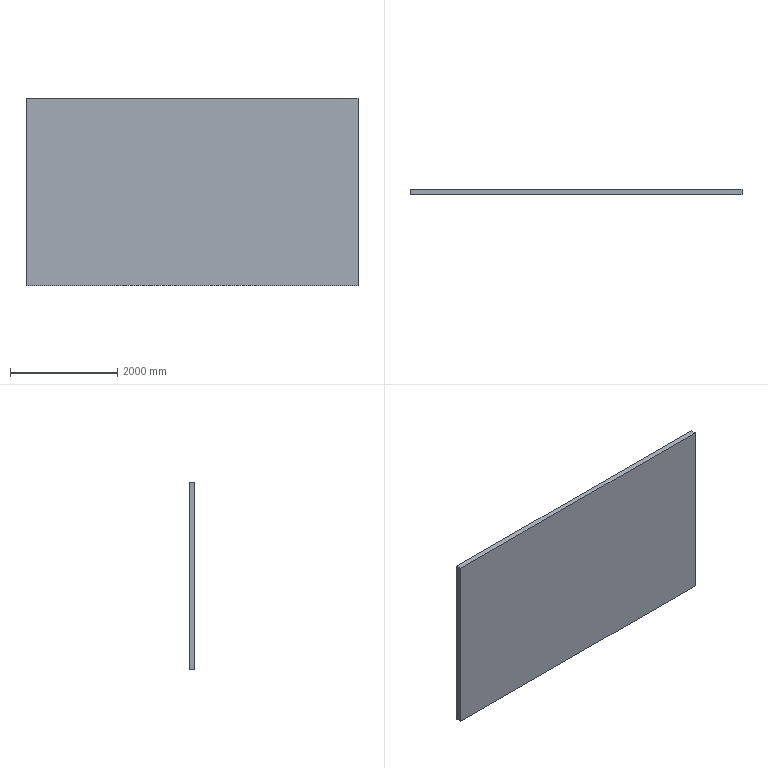Part | SolidWorks | features Cut 1, Extrusion 1 | 1 solid | 6 faces | box 6200 x 100 x 3500 mm | volume 2170000000 mm3 | plane 6
STEP:
#1=CARTESIAN_POINT('',(2800.,0.,-2400.));
#2=VERTEX_POINT('',#1);
#3=CARTESIAN_POINT('',(2800.,100.,-2400.));
#4=VERTEX_POINT('',#3);
#5=CARTESIAN_POINT('',(2800.,0.,-2400.));
#6=DIRECTION('',(0.,1.,0.));
#7=VECTOR('',#6,1000.);
#8=LINE('',#5,#7);
#9=EDGE_CURVE('',#2,#4,#8,.T.);
#10=ORIENTED_EDGE('',*,*,#9,.F.);
#11=CARTESIAN_POINT('',(-3400.,0.,-2400.));
#12=VERTEX_POINT('',#11);
#13=CARTESIAN_POINT('',(-3400.,0.,-2400.));
#14=DIRECTION('',(-1.,0.,0.));
#15=VECTOR('',#14,1000.);
#16=LINE('',#13,#15);
#17=EDGE_CURVE('',#2,#12,#16,.T.);
#18=ORIENTED_EDGE('',*,*,#17,.T.);
#19=CARTESIAN_POINT('',(-3400.,100.,-2400.));
#20=VERTEX_POINT('',#19);
#21=CARTESIAN_POINT('',(-3400.,100.,-2400.));
#22=DIRECTION('',(0.,-1.,0.));
#23=VECTOR('',#22,1000.);
#24=LINE('',#21,#23);
#25=EDGE_CURVE('',#20,#12,#24,.T.);
#26=ORIENTED_EDGE('',*,*,#25,.F.);
#27=CARTESIAN_POINT('',(-3400.,100.,-2400.));
#28=DIRECTION('',(-1.,0.,0.));
#29=VECTOR('',#28,1000.);
#30=LINE('',#27,#29);
#31=EDGE_CURVE('',#4,#20,#30,.T.);
#32=ORIENTED_EDGE('',*,*,#31,.F.);
#33=EDGE_LOOP('',(#10,#18,#26,#32));
#34=FACE_OUTER_BOUND('',#33,.T.);
#35=CARTESIAN_POINT('',(-3400.,100.,-2400.));
#36=DIRECTION('',(0.,0.,1.));
#37=DIRECTION('',(1.,0.,0.));
#38=AXIS2_PLACEMENT_3D('',#35,#36,#37);
#39=PLANE('',#38);
#40=ADVANCED_FACE('',(#34),#39,.F.);
#41=CARTESIAN_POINT('',(-3400.,0.,1100.));
#42=VERTEX_POINT('',#41);
#43=CARTESIAN_POINT('',(-3400.,100.,1100.));
#44=VERTEX_POINT('',#43);
#45=CARTESIAN_POINT('',(-3400.,0.,1100.));
#46=DIRECTION('',(0.,1.,0.));
#47=VECTOR('',#46,1000.);
#48=LINE('',#45,#47);
#49=EDGE_CURVE('',#42,#44,#48,.T.);
#50=ORIENTED_EDGE('',*,*,#49,.T.);
#51=CARTESIAN_POINT('',(-3400.,100.,-2400.));
#52=DIRECTION('',(0.,0.,1.));
#53=VECTOR('',#52,1000.);
#54=LINE('',#51,#53);
#55=EDGE_CURVE('',#20,#44,#54,.T.);
#56=ORIENTED_EDGE('',*,*,#55,.F.);
#57=ORIENTED_EDGE('',*,*,#25,.T.);
#58=CARTESIAN_POINT('',(-3400.,0.,-2400.));
#59=DIRECTION('',(0.,0.,1.));
#60=VECTOR('',#59,1000.);
#61=LINE('',#58,#60);
#62=EDGE_CURVE('',#12,#42,#61,.T.);
#63=ORIENTED_EDGE('',*,*,#62,.T.);
#64=EDGE_LOOP('',(#50,#56,#57,#63));
#65=FACE_OUTER_BOUND('',#64,.T.);
#66=CARTESIAN_POINT('',(-3400.,100.,-2400.));
#67=DIRECTION('',(1.,0.,0.));
#68=DIRECTION('',(0.,0.,-1.));
#69=AXIS2_PLACEMENT_3D('',#66,#67,#68);
#70=PLANE('',#69);
#71=ADVANCED_FACE('',(#65),#70,.F.);
#72=CARTESIAN_POINT('',(2800.,100.,1100.));
#73=VERTEX_POINT('',#72);
#74=CARTESIAN_POINT('',(-3400.,100.,1100.));
#75=DIRECTION('',(1.,0.,0.));
#76=VECTOR('',#75,1000.);
#77=LINE('',#74,#76);
#78=EDGE_CURVE('',#44,#73,#77,.T.);
#79=ORIENTED_EDGE('',*,*,#78,.T.);
#80=CARTESIAN_POINT('',(2800.,100.,-2400.));
#81=DIRECTION('',(0.,0.,-1.));
#82=VECTOR('',#81,1000.);
#83=LINE('',#80,#82);
#84=EDGE_CURVE('',#73,#4,#83,.T.);
#85=ORIENTED_EDGE('',*,*,#84,.T.);
#86=ORIENTED_EDGE('',*,*,#31,.T.);
#87=ORIENTED_EDGE('',*,*,#55,.T.);
#88=EDGE_LOOP('',(#79,#85,#86,#87));
#89=FACE_OUTER_BOUND('',#88,.T.);
#90=CARTESIAN_POINT('',(0.,100.,0.));
#91=DIRECTION('',(0.,1.,0.));
#92=DIRECTION('',(0.,0.,1.));
#93=AXIS2_PLACEMENT_3D('',#90,#91,#92);
#94=PLANE('',#93);
#95=ADVANCED_FACE('',(#89),#94,.T.);
#96=CARTESIAN_POINT('',(2800.,0.,1100.));
#97=VERTEX_POINT('',#96);
#98=CARTESIAN_POINT('',(2800.,0.,-2400.));
#99=DIRECTION('',(0.,0.,-1.));
#100=VECTOR('',#99,1000.);
#101=LINE('',#98,#100);
#102=EDGE_CURVE('',#97,#2,#101,.T.);
#103=ORIENTED_EDGE('',*,*,#102,.F.);
#104=CARTESIAN_POINT('',(-3400.,0.,1100.));
#105=DIRECTION('',(1.,0.,0.));
#106=VECTOR('',#105,1000.);
#107=LINE('',#104,#106);
#108=EDGE_CURVE('',#42,#97,#107,.T.);
#109=ORIENTED_EDGE('',*,*,#108,.F.);
#110=ORIENTED_EDGE('',*,*,#62,.F.);
#111=ORIENTED_EDGE('',*,*,#17,.F.);
#112=EDGE_LOOP('',(#103,#109,#110,#111));
#113=FACE_OUTER_BOUND('',#112,.T.);
#114=CARTESIAN_POINT('',(0.,0.,0.));
#115=DIRECTION('',(0.,1.,0.));
#116=DIRECTION('',(0.,0.,1.));
#117=AXIS2_PLACEMENT_3D('',#114,#115,#116);
#118=PLANE('',#117);
#119=ADVANCED_FACE('',(#113),#118,.F.);
#120=ORIENTED_EDGE('',*,*,#84,.F.);
#121=CARTESIAN_POINT('',(2800.,0.,1100.));
#122=DIRECTION('',(0.,1.,0.));
#123=VECTOR('',#122,1000.);
#124=LINE('',#121,#123);
#125=EDGE_CURVE('',#97,#73,#124,.T.);
#126=ORIENTED_EDGE('',*,*,#125,.F.);
#127=ORIENTED_EDGE('',*,*,#102,.T.);
#128=ORIENTED_EDGE('',*,*,#9,.T.);
#129=EDGE_LOOP('',(#120,#126,#127,#128));
#130=FACE_OUTER_BOUND('',#129,.T.);
#131=CARTESIAN_POINT('',(2800.,0.,-2400.));
#132=DIRECTION('',(1.,0.,0.));
#133=DIRECTION('',(0.,0.,-1.));
#134=AXIS2_PLACEMENT_3D('',#131,#132,#133);
#135=PLANE('',#134);
#136=ADVANCED_FACE('',(#130),#135,.T.);
#137=ORIENTED_EDGE('',*,*,#78,.F.);
#138=ORIENTED_EDGE('',*,*,#49,.F.);
#139=ORIENTED_EDGE('',*,*,#108,.T.);
#140=ORIENTED_EDGE('',*,*,#125,.T.);
#141=EDGE_LOOP('',(#137,#138,#139,#140));
#142=FACE_OUTER_BOUND('',#141,.T.);
#143=CARTESIAN_POINT('',(-3400.,0.,1100.));
#144=DIRECTION('',(0.,0.,1.));
#145=DIRECTION('',(1.,0.,0.));
#146=AXIS2_PLACEMENT_3D('',#143,#144,#145);
#147=PLANE('',#146);
#148=ADVANCED_FACE('',(#142),#147,.T.);
#149=CLOSED_SHELL('',(#40,#71,#95,#119,#136,#148));
#150=MANIFOLD_SOLID_BREP('',#149);
#151=CARTESIAN_POINT('',(0.,0.,0.));
#152=DIRECTION('',(0.,0.,1.));
#153=DIRECTION('',(1.,0.,0.));
#154=AXIS2_PLACEMENT_3D('',#151,#152,#153);
#155=(LENGTH_UNIT()NAMED_UNIT(*)SI_UNIT(.MILLI.,.METRE.));
#156=UNCERTAINTY_MEASURE_WITH_UNIT(LENGTH_MEASURE(0.00001),#155,'','');
#157=(NAMED_UNIT(*)PLANE_ANGLE_UNIT()SI_UNIT($,.RADIAN.));
#158=(NAMED_UNIT(*)SI_UNIT($,.STERADIAN.)SOLID_ANGLE_UNIT());
#159=(GEOMETRIC_REPRESENTATION_CONTEXT(3)GLOBAL_UNCERTAINTY_ASSIGNED_CONTEXT((#156))GLOBAL_UNIT_ASSIGNED_CONTEXT((#155,#157,#158))REPRESENTATION_CONTEXT('',''));
#160=ADVANCED_BREP_SHAPE_REPRESENTATION('',(#150,#154),#159);